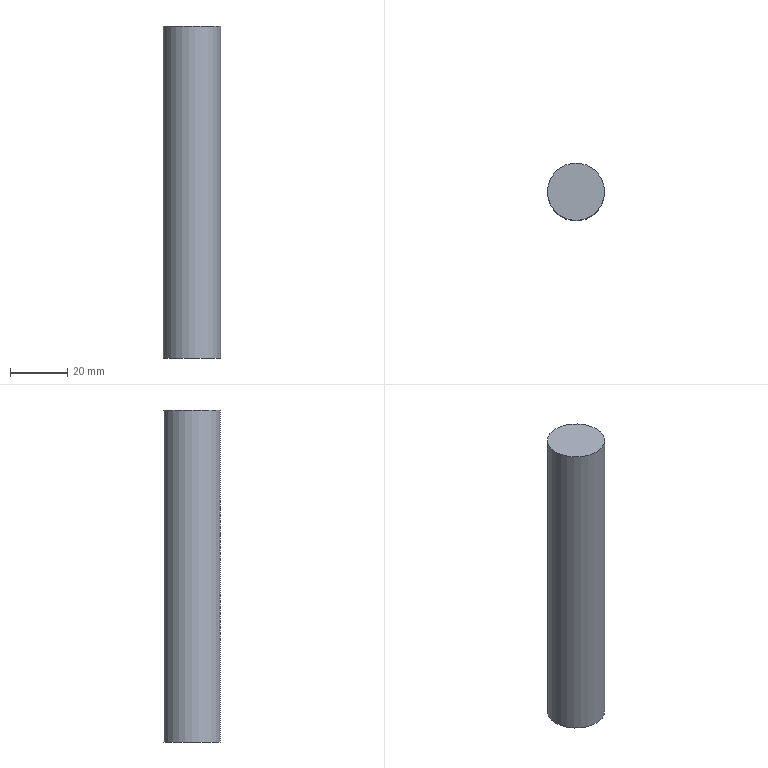Part | NX | features solid 2 | 1 solid | 3 faces | box 20 x 20 x 116 mm | volume 36442 mm3 | plane 2 | cylinder 1 | commonest cylinder face diameters 20 x1
STEP:
#1=CARTESIAN_POINT('',(-506.,9.,-174.));
#2=VERTEX_POINT('',#1);
#3=CARTESIAN_POINT('',(-516.,9.,-174.));
#4=DIRECTION('',(0.,0.,1.));
#5=DIRECTION('',(1.,0.,0.));
#6=AXIS2_PLACEMENT_3D('',#3,#4,#5);
#7=CIRCLE('',#6,10.);
#8=EDGE_CURVE('',#2,#2,#7,.T.);
#9=ORIENTED_EDGE('',*,*,#8,.T.);
#10=EDGE_LOOP('',(#9));
#11=FACE_BOUND('',#10,.T.);
#12=CARTESIAN_POINT('',(-506.,9.,-58.));
#13=VERTEX_POINT('',#12);
#14=CARTESIAN_POINT('',(-516.,9.,-58.));
#15=DIRECTION('',(0.,0.,1.));
#16=DIRECTION('',(1.,0.,0.));
#17=AXIS2_PLACEMENT_3D('',#14,#15,#16);
#18=CIRCLE('',#17,10.);
#19=EDGE_CURVE('',#13,#13,#18,.T.);
#20=ORIENTED_EDGE('',*,*,#19,.F.);
#21=EDGE_LOOP('',(#20));
#22=FACE_BOUND('',#21,.T.);
#23=CARTESIAN_POINT('',(-516.,9.,-186.));
#24=DIRECTION('',(0.,0.,1.));
#25=DIRECTION('',(1.,0.,0.));
#26=AXIS2_PLACEMENT_3D('',#23,#24,#25);
#27=CYLINDRICAL_SURFACE('',#26,10.);
#28=ADVANCED_FACE('',(#11,#22),#27,.T.);
#29=ORIENTED_EDGE('',*,*,#19,.T.);
#30=EDGE_LOOP('',(#29));
#31=FACE_BOUND('',#30,.T.);
#32=CARTESIAN_POINT('',(-516.,9.,-58.));
#33=DIRECTION('',(0.,0.,1.));
#34=DIRECTION('',(1.,0.,0.));
#35=AXIS2_PLACEMENT_3D('',#32,#33,#34);
#36=PLANE('',#35);
#37=ADVANCED_FACE('',(#31),#36,.T.);
#38=ORIENTED_EDGE('',*,*,#8,.F.);
#39=EDGE_LOOP('',(#38));
#40=FACE_BOUND('',#39,.T.);
#41=CARTESIAN_POINT('',(-516.,9.,-174.));
#42=DIRECTION('',(0.,0.,1.));
#43=DIRECTION('',(1.,0.,0.));
#44=AXIS2_PLACEMENT_3D('',#41,#42,#43);
#45=PLANE('',#44);
#46=ADVANCED_FACE('',(#40),#45,.F.);
#47=CLOSED_SHELL('',(#28,#37,#46));
#48=MANIFOLD_SOLID_BREP('',#47);
#49=(LENGTH_UNIT()NAMED_UNIT(*)SI_UNIT(.MILLI.,.METRE.));
#50=UNCERTAINTY_MEASURE_WITH_UNIT(LENGTH_MEASURE(0.00001),#49,'','');
#51=(NAMED_UNIT(*)PLANE_ANGLE_UNIT()SI_UNIT($,.RADIAN.));
#52=(NAMED_UNIT(*)SI_UNIT($,.STERADIAN.)SOLID_ANGLE_UNIT());
#53=(GEOMETRIC_REPRESENTATION_CONTEXT(3)GLOBAL_UNCERTAINTY_ASSIGNED_CONTEXT((#50))GLOBAL_UNIT_ASSIGNED_CONTEXT((#49,#51,#52))REPRESENTATION_CONTEXT('',''));
#54=ADVANCED_BREP_SHAPE_REPRESENTATION('',(#48),#53);